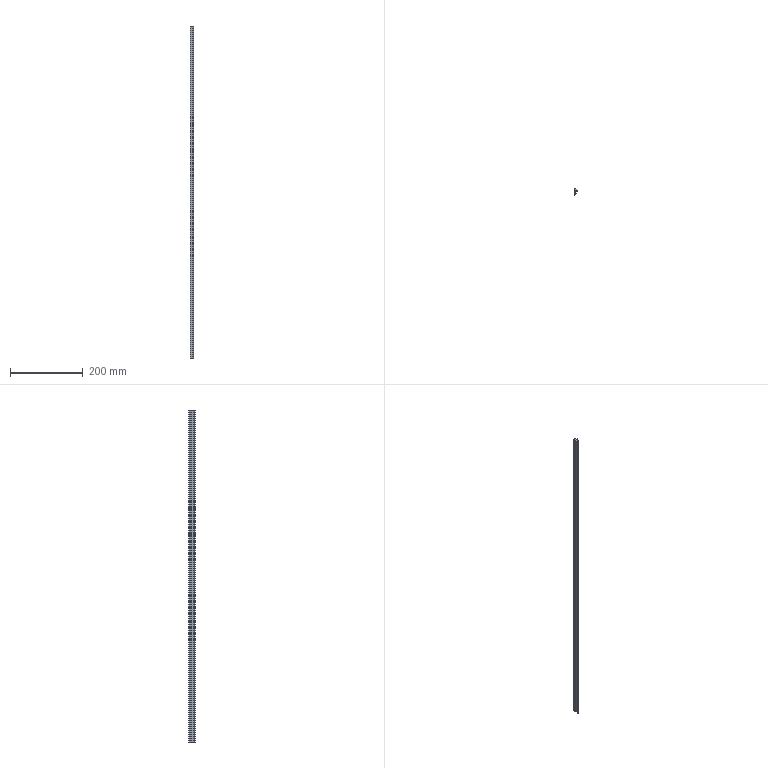Part | SolidWorks | features BaseBody 1, MoveFace 1 | 1 solid | 20 faces | box 10.8 x 17.5 x 915 mm | volume 72103 mm3 | cylinder 11 | plane 9 | commonest cylinder face diameters 1.6 x2 14 x2 0.4 x1 0.6 x1 0.8 x1 2.6 x1
STEP:
#1=CARTESIAN_POINT('',(-3.236,-11.055,815.));
#2=VERTEX_POINT('',#1);
#3=CARTESIAN_POINT('',(-4.3,-10.3,815.));
#4=VERTEX_POINT('',#3);
#5=CARTESIAN_POINT('',(-3.5,-10.3,815.));
#6=DIRECTION('',(0.,0.,-1.));
#7=DIRECTION('',(1.,0.,0.));
#8=AXIS2_PLACEMENT_3D('',#5,#6,#7);
#9=CIRCLE('',#8,0.8);
#10=EDGE_CURVE('',#2,#4,#9,.T.);
#11=ORIENTED_EDGE('',*,*,#10,.T.);
#12=CARTESIAN_POINT('',(-4.3,-10.3,-100.));
#13=VERTEX_POINT('',#12);
#14=CARTESIAN_POINT('',(-4.3,-10.3,-100.));
#15=DIRECTION('',(0.,0.,-1.));
#16=VECTOR('',#15,1000.);
#17=LINE('',#14,#16);
#18=EDGE_CURVE('',#4,#13,#17,.T.);
#19=ORIENTED_EDGE('',*,*,#18,.T.);
#20=CARTESIAN_POINT('',(-3.236,-11.055,-100.));
#21=VERTEX_POINT('',#20);
#22=CARTESIAN_POINT('',(-3.5,-10.3,-100.));
#23=DIRECTION('',(0.,0.,1.));
#24=DIRECTION('',(-1.,0.,0.));
#25=AXIS2_PLACEMENT_3D('',#22,#23,#24);
#26=CIRCLE('',#25,0.8);
#27=EDGE_CURVE('',#13,#21,#26,.T.);
#28=ORIENTED_EDGE('',*,*,#27,.T.);
#29=CARTESIAN_POINT('',(-3.236,-11.055,-100.));
#30=DIRECTION('',(0.,0.,-1.));
#31=VECTOR('',#30,1000.);
#32=LINE('',#29,#31);
#33=EDGE_CURVE('',#2,#21,#32,.T.);
#34=ORIENTED_EDGE('',*,*,#33,.F.);
#35=EDGE_LOOP('',(#11,#19,#28,#34));
#36=FACE_OUTER_BOUND('',#35,.T.);
#37=CARTESIAN_POINT('',(-3.5,-10.3,-100.));
#38=DIRECTION('',(0.,0.,-1.));
#39=DIRECTION('',(-1.,0.,0.));
#40=AXIS2_PLACEMENT_3D('',#37,#38,#39);
#41=CYLINDRICAL_SURFACE('',#40,0.8);
#42=ADVANCED_FACE('',(#36),#41,.T.);
#43=CARTESIAN_POINT('',(1.184,-6.397,-100.));
#44=VERTEX_POINT('',#43);
#45=CARTESIAN_POINT('',(-5.702,-4.29,-100.));
#46=DIRECTION('',(0.,0.,1.));
#47=DIRECTION('',(-1.,0.,0.));
#48=AXIS2_PLACEMENT_3D('',#45,#46,#47);
#49=CIRCLE('',#48,7.201);
#50=EDGE_CURVE('',#21,#44,#49,.T.);
#51=ORIENTED_EDGE('',*,*,#50,.T.);
#52=CARTESIAN_POINT('',(1.184,-6.397,815.));
#53=VERTEX_POINT('',#52);
#54=CARTESIAN_POINT('',(1.184,-6.397,-100.));
#55=DIRECTION('',(0.,0.,1.));
#56=VECTOR('',#55,1000.);
#57=LINE('',#54,#56);
#58=EDGE_CURVE('',#44,#53,#57,.T.);
#59=ORIENTED_EDGE('',*,*,#58,.T.);
#60=CARTESIAN_POINT('',(-5.702,-4.29,815.));
#61=DIRECTION('',(0.,0.,-1.));
#62=DIRECTION('',(1.,0.,0.));
#63=AXIS2_PLACEMENT_3D('',#60,#61,#62);
#64=CIRCLE('',#63,7.201);
#65=EDGE_CURVE('',#53,#2,#64,.T.);
#66=ORIENTED_EDGE('',*,*,#65,.T.);
#67=ORIENTED_EDGE('',*,*,#33,.T.);
#68=EDGE_LOOP('',(#51,#59,#66,#67));
#69=FACE_OUTER_BOUND('',#68,.T.);
#70=CARTESIAN_POINT('',(-5.702,-4.29,-100.));
#71=DIRECTION('',(0.,0.,-1.));
#72=DIRECTION('',(-1.,0.,0.));
#73=AXIS2_PLACEMENT_3D('',#70,#71,#72);
#74=CYLINDRICAL_SURFACE('',#73,7.201);
#75=ADVANCED_FACE('',(#69),#74,.T.);
#76=CARTESIAN_POINT('',(0.9,-6.,-100.));
#77=VERTEX_POINT('',#76);
#78=CARTESIAN_POINT('',(0.9,-6.3,-100.));
#79=DIRECTION('',(0.,0.,1.));
#80=DIRECTION('',(-1.,0.,0.));
#81=AXIS2_PLACEMENT_3D('',#78,#79,#80);
#82=CIRCLE('',#81,0.3);
#83=EDGE_CURVE('',#44,#77,#82,.T.);
#84=ORIENTED_EDGE('',*,*,#83,.T.);
#85=CARTESIAN_POINT('',(0.9,-6.,815.));
#86=VERTEX_POINT('',#85);
#87=CARTESIAN_POINT('',(0.9,-6.,-100.));
#88=DIRECTION('',(0.,0.,1.));
#89=VECTOR('',#88,1000.);
#90=LINE('',#87,#89);
#91=EDGE_CURVE('',#77,#86,#90,.T.);
#92=ORIENTED_EDGE('',*,*,#91,.T.);
#93=CARTESIAN_POINT('',(0.9,-6.3,815.));
#94=DIRECTION('',(0.,0.,-1.));
#95=DIRECTION('',(1.,0.,0.));
#96=AXIS2_PLACEMENT_3D('',#93,#94,#95);
#97=CIRCLE('',#96,0.3);
#98=EDGE_CURVE('',#86,#53,#97,.T.);
#99=ORIENTED_EDGE('',*,*,#98,.T.);
#100=ORIENTED_EDGE('',*,*,#58,.F.);
#101=EDGE_LOOP('',(#84,#92,#99,#100));
#102=FACE_OUTER_BOUND('',#101,.T.);
#103=CARTESIAN_POINT('',(0.9,-6.3,-100.));
#104=DIRECTION('',(0.,0.,-1.));
#105=DIRECTION('',(-1.,0.,0.));
#106=AXIS2_PLACEMENT_3D('',#103,#104,#105);
#107=CYLINDRICAL_SURFACE('',#106,0.3);
#108=ADVANCED_FACE('',(#102),#107,.T.);
#109=CARTESIAN_POINT('',(-2.5,-0.5,-100.));
#110=VERTEX_POINT('',#109);
#111=CARTESIAN_POINT('',(-2.5,-6.153,-100.));
#112=VERTEX_POINT('',#111);
#113=CARTESIAN_POINT('',(-2.5,-6.397,-100.));
#114=DIRECTION('',(0.,-1.,0.));
#115=VECTOR('',#114,1000.);
#116=LINE('',#113,#115);
#117=EDGE_CURVE('',#110,#112,#116,.T.);
#118=ORIENTED_EDGE('',*,*,#117,.F.);
#119=CARTESIAN_POINT('',(-4.2,1.695,-100.));
#120=VERTEX_POINT('',#119);
#121=CARTESIAN_POINT('',(-1.701,1.875,-100.));
#122=DIRECTION('',(0.,0.,1.));
#123=DIRECTION('',(-1.,0.,0.));
#124=AXIS2_PLACEMENT_3D('',#121,#122,#123);
#125=CIRCLE('',#124,2.506);
#126=EDGE_CURVE('',#120,#110,#125,.T.);
#127=ORIENTED_EDGE('',*,*,#126,.F.);
#128=CARTESIAN_POINT('',(-4.2,5.1,-100.));
#129=VERTEX_POINT('',#128);
#130=CARTESIAN_POINT('',(-4.2,-6.397,-100.));
#131=DIRECTION('',(0.,-1.,0.));
#132=VECTOR('',#131,1000.);
#133=LINE('',#130,#132);
#134=EDGE_CURVE('',#129,#120,#133,.T.);
#135=ORIENTED_EDGE('',*,*,#134,.F.);
#136=CARTESIAN_POINT('',(-2.892,6.4,-100.));
#137=VERTEX_POINT('',#136);
#138=CARTESIAN_POINT('',(-2.9,5.1,-100.));
#139=DIRECTION('',(0.,0.,1.));
#140=DIRECTION('',(-1.,0.,0.));
#141=AXIS2_PLACEMENT_3D('',#138,#139,#140);
#142=CIRCLE('',#141,1.3);
#143=EDGE_CURVE('',#137,#129,#142,.T.);
#144=ORIENTED_EDGE('',*,*,#143,.F.);
#145=CARTESIAN_POINT('',(0.5,5.5,-100.));
#146=VERTEX_POINT('',#145);
#147=CARTESIAN_POINT('',(-2.934,-0.5999,-100.));
#148=DIRECTION('',(0.,0.,1.));
#149=DIRECTION('',(-1.,0.,0.));
#150=AXIS2_PLACEMENT_3D('',#147,#148,#149);
#151=CIRCLE('',#150,7.);
#152=EDGE_CURVE('',#146,#137,#151,.T.);
#153=ORIENTED_EDGE('',*,*,#152,.F.);
#154=CARTESIAN_POINT('',(5.5,1.7,-100.));
#155=VERTEX_POINT('',#154);
#156=CARTESIAN_POINT('',(5.5,1.7,-100.));
#157=DIRECTION('',(-0.7962,0.6051,0.));
#158=VECTOR('',#157,1000.);
#159=LINE('',#156,#158);
#160=EDGE_CURVE('',#155,#146,#159,.T.);
#161=ORIENTED_EDGE('',*,*,#160,.F.);
#162=CARTESIAN_POINT('',(6.458,-0.2215,-100.));
#163=VERTEX_POINT('',#162);
#164=CARTESIAN_POINT('',(6.458,-0.2215,-100.));
#165=DIRECTION('',(-0.4462,0.8949,0.));
#166=VECTOR('',#165,1000.);
#167=LINE('',#164,#166);
#168=EDGE_CURVE('',#163,#155,#167,.T.);
#169=ORIENTED_EDGE('',*,*,#168,.F.);
#170=CARTESIAN_POINT('',(5.895,-0.7433,-100.));
#171=VERTEX_POINT('',#170);
#172=CARTESIAN_POINT('',(6.1,-0.4,-100.));
#173=DIRECTION('',(0.,0.,1.));
#174=DIRECTION('',(-1.,0.,0.));
#175=AXIS2_PLACEMENT_3D('',#172,#173,#174);
#176=CIRCLE('',#175,0.4);
#177=EDGE_CURVE('',#171,#163,#176,.T.);
#178=ORIENTED_EDGE('',*,*,#177,.F.);
#179=CARTESIAN_POINT('',(3.,0.,-100.));
#180=VERTEX_POINT('',#179);
#181=CARTESIAN_POINT('',(2.746,-6.995,-100.));
#182=DIRECTION('',(0.,0.,-1.));
#183=DIRECTION('',(-1.,0.,0.));
#184=AXIS2_PLACEMENT_3D('',#181,#182,#183);
#185=CIRCLE('',#184,7.);
#186=EDGE_CURVE('',#180,#171,#185,.T.);
#187=ORIENTED_EDGE('',*,*,#186,.F.);
#188=CARTESIAN_POINT('',(0.,0.,-100.));
#189=VERTEX_POINT('',#188);
#190=CARTESIAN_POINT('',(-6.814,0.,-100.));
#191=DIRECTION('',(1.,0.,0.));
#192=VECTOR('',#191,1000.);
#193=LINE('',#190,#192);
#194=EDGE_CURVE('',#189,#180,#193,.T.);
#195=ORIENTED_EDGE('',*,*,#194,.F.);
#196=CARTESIAN_POINT('',(0.,-5.8,-100.));
#197=VERTEX_POINT('',#196);
#198=CARTESIAN_POINT('',(0.,-6.397,-100.));
#199=DIRECTION('',(0.,1.,0.));
#200=VECTOR('',#199,1000.);
#201=LINE('',#198,#200);
#202=EDGE_CURVE('',#197,#189,#201,.T.);
#203=ORIENTED_EDGE('',*,*,#202,.F.);
#204=CARTESIAN_POINT('',(0.2,-6.,-100.));
#205=VERTEX_POINT('',#204);
#206=CARTESIAN_POINT('',(0.2,-5.8,-100.));
#207=DIRECTION('',(0.,0.,1.));
#208=DIRECTION('',(-1.,0.,0.));
#209=AXIS2_PLACEMENT_3D('',#206,#207,#208);
#210=CIRCLE('',#209,0.2);
#211=EDGE_CURVE('',#197,#205,#210,.T.);
#212=ORIENTED_EDGE('',*,*,#211,.T.);
#213=CARTESIAN_POINT('',(-6.814,-6.,-100.));
#214=DIRECTION('',(-1.,0.,0.));
#215=VECTOR('',#214,1000.);
#216=LINE('',#213,#215);
#217=EDGE_CURVE('',#77,#205,#216,.T.);
#218=ORIENTED_EDGE('',*,*,#217,.F.);
#219=ORIENTED_EDGE('',*,*,#83,.F.);
#220=ORIENTED_EDGE('',*,*,#50,.F.);
#221=ORIENTED_EDGE('',*,*,#27,.F.);
#222=CARTESIAN_POINT('',(-3.998,-9.674,-100.));
#223=VERTEX_POINT('',#222);
#224=CARTESIAN_POINT('',(-3.5,-10.3,-100.));
#225=DIRECTION('',(0.,0.,1.));
#226=DIRECTION('',(-1.,0.,0.));
#227=AXIS2_PLACEMENT_3D('',#224,#225,#226);
#228=CIRCLE('',#227,0.8);
#229=EDGE_CURVE('',#223,#13,#228,.T.);
#230=ORIENTED_EDGE('',*,*,#229,.F.);
#231=CARTESIAN_POINT('',(-6.814,-6.397,-100.));
#232=DIRECTION('',(0.,0.,-1.));
#233=DIRECTION('',(-1.,0.,0.));
#234=AXIS2_PLACEMENT_3D('',#231,#232,#233);
#235=CIRCLE('',#234,4.321);
#236=EDGE_CURVE('',#112,#223,#235,.T.);
#237=ORIENTED_EDGE('',*,*,#236,.F.);
#238=EDGE_LOOP('',(#118,#127,#135,#144,#153,#161,#169,#178,#187,#195,#203,#212,#218,#219,#220,#221,#230,#237));
#239=FACE_OUTER_BOUND('',#238,.T.);
#240=CARTESIAN_POINT('',(-6.814,-6.397,-100.));
#241=DIRECTION('',(0.,0.,1.));
#242=DIRECTION('',(1.,0.,0.));
#243=AXIS2_PLACEMENT_3D('',#240,#241,#242);
#244=PLANE('',#243);
#245=ADVANCED_FACE('',(#239),#244,.F.);
#246=ORIENTED_EDGE('',*,*,#18,.F.);
#247=CARTESIAN_POINT('',(-3.998,-9.674,815.));
#248=VERTEX_POINT('',#247);
#249=CARTESIAN_POINT('',(-3.5,-10.3,815.));
#250=DIRECTION('',(0.,0.,-1.));
#251=DIRECTION('',(1.,0.,0.));
#252=AXIS2_PLACEMENT_3D('',#249,#250,#251);
#253=CIRCLE('',#252,0.8);
#254=EDGE_CURVE('',#4,#248,#253,.T.);
#255=ORIENTED_EDGE('',*,*,#254,.T.);
#256=CARTESIAN_POINT('',(-3.998,-9.674,-100.));
#257=DIRECTION('',(0.,0.,-1.));
#258=VECTOR('',#257,1000.);
#259=LINE('',#256,#258);
#260=EDGE_CURVE('',#248,#223,#259,.T.);
#261=ORIENTED_EDGE('',*,*,#260,.T.);
#262=ORIENTED_EDGE('',*,*,#229,.T.);
#263=EDGE_LOOP('',(#246,#255,#261,#262));
#264=FACE_OUTER_BOUND('',#263,.T.);
#265=CARTESIAN_POINT('',(-3.5,-10.3,-100.));
#266=DIRECTION('',(0.,0.,-1.));
#267=DIRECTION('',(-1.,0.,0.));
#268=AXIS2_PLACEMENT_3D('',#265,#266,#267);
#269=CYLINDRICAL_SURFACE('',#268,0.8);
#270=ADVANCED_FACE('',(#264),#269,.T.);
#271=CARTESIAN_POINT('',(-4.2,1.695,815.));
#272=VERTEX_POINT('',#271);
#273=CARTESIAN_POINT('',(-2.5,-0.5,815.));
#274=VERTEX_POINT('',#273);
#275=CARTESIAN_POINT('',(-1.701,1.875,815.));
#276=DIRECTION('',(0.,0.,1.));
#277=DIRECTION('',(1.,0.,0.));
#278=AXIS2_PLACEMENT_3D('',#275,#276,#277);
#279=CIRCLE('',#278,2.506);
#280=EDGE_CURVE('',#272,#274,#279,.T.);
#281=ORIENTED_EDGE('',*,*,#280,.T.);
#282=CARTESIAN_POINT('',(-2.5,-6.153,815.));
#283=VERTEX_POINT('',#282);
#284=CARTESIAN_POINT('',(-2.5,-6.397,815.));
#285=DIRECTION('',(0.,-1.,0.));
#286=VECTOR('',#285,1000.);
#287=LINE('',#284,#286);
#288=EDGE_CURVE('',#274,#283,#287,.T.);
#289=ORIENTED_EDGE('',*,*,#288,.T.);
#290=CARTESIAN_POINT('',(-6.814,-6.397,815.));
#291=DIRECTION('',(0.,0.,-1.));
#292=DIRECTION('',(1.,0.,0.));
#293=AXIS2_PLACEMENT_3D('',#290,#291,#292);
#294=CIRCLE('',#293,4.321);
#295=EDGE_CURVE('',#283,#248,#294,.T.);
#296=ORIENTED_EDGE('',*,*,#295,.T.);
#297=ORIENTED_EDGE('',*,*,#254,.F.);
#298=ORIENTED_EDGE('',*,*,#10,.F.);
#299=ORIENTED_EDGE('',*,*,#65,.F.);
#300=ORIENTED_EDGE('',*,*,#98,.F.);
#301=CARTESIAN_POINT('',(0.2,-6.,815.));
#302=VERTEX_POINT('',#301);
#303=CARTESIAN_POINT('',(-6.814,-6.,815.));
#304=DIRECTION('',(-1.,0.,0.));
#305=VECTOR('',#304,1000.);
#306=LINE('',#303,#305);
#307=EDGE_CURVE('',#86,#302,#306,.T.);
#308=ORIENTED_EDGE('',*,*,#307,.T.);
#309=CARTESIAN_POINT('',(0.,-5.8,815.));
#310=VERTEX_POINT('',#309);
#311=CARTESIAN_POINT('',(0.2,-5.8,815.));
#312=DIRECTION('',(0.,0.,-1.));
#313=DIRECTION('',(1.,0.,0.));
#314=AXIS2_PLACEMENT_3D('',#311,#312,#313);
#315=CIRCLE('',#314,0.2);
#316=EDGE_CURVE('',#302,#310,#315,.T.);
#317=ORIENTED_EDGE('',*,*,#316,.T.);
#318=CARTESIAN_POINT('',(0.,0.,815.));
#319=VERTEX_POINT('',#318);
#320=CARTESIAN_POINT('',(0.,-6.397,815.));
#321=DIRECTION('',(0.,1.,0.));
#322=VECTOR('',#321,1000.);
#323=LINE('',#320,#322);
#324=EDGE_CURVE('',#310,#319,#323,.T.);
#325=ORIENTED_EDGE('',*,*,#324,.T.);
#326=CARTESIAN_POINT('',(3.,0.,815.));
#327=VERTEX_POINT('',#326);
#328=CARTESIAN_POINT('',(-6.814,0.,815.));
#329=DIRECTION('',(1.,0.,0.));
#330=VECTOR('',#329,1000.);
#331=LINE('',#328,#330);
#332=EDGE_CURVE('',#319,#327,#331,.T.);
#333=ORIENTED_EDGE('',*,*,#332,.T.);
#334=CARTESIAN_POINT('',(5.895,-0.7433,815.));
#335=VERTEX_POINT('',#334);
#336=CARTESIAN_POINT('',(2.746,-6.995,815.));
#337=DIRECTION('',(0.,0.,-1.));
#338=DIRECTION('',(1.,0.,0.));
#339=AXIS2_PLACEMENT_3D('',#336,#337,#338);
#340=CIRCLE('',#339,7.);
#341=EDGE_CURVE('',#327,#335,#340,.T.);
#342=ORIENTED_EDGE('',*,*,#341,.T.);
#343=CARTESIAN_POINT('',(6.458,-0.2215,815.));
#344=VERTEX_POINT('',#343);
#345=CARTESIAN_POINT('',(6.1,-0.4,815.));
#346=DIRECTION('',(0.,0.,-1.));
#347=DIRECTION('',(1.,0.,0.));
#348=AXIS2_PLACEMENT_3D('',#345,#346,#347);
#349=CIRCLE('',#348,0.4);
#350=EDGE_CURVE('',#344,#335,#349,.T.);
#351=ORIENTED_EDGE('',*,*,#350,.F.);
#352=CARTESIAN_POINT('',(5.5,1.7,815.));
#353=VERTEX_POINT('',#352);
#354=CARTESIAN_POINT('',(6.282,0.1323,815.));
#355=DIRECTION('',(-0.4462,0.8949,0.));
#356=VECTOR('',#355,1000.);
#357=LINE('',#354,#356);
#358=EDGE_CURVE('',#344,#353,#357,.T.);
#359=ORIENTED_EDGE('',*,*,#358,.T.);
#360=CARTESIAN_POINT('',(0.5,5.5,815.));
#361=VERTEX_POINT('',#360);
#362=CARTESIAN_POINT('',(1.595,4.668,815.));
#363=DIRECTION('',(-0.7962,0.6051,0.));
#364=VECTOR('',#363,1000.);
#365=LINE('',#362,#364);
#366=EDGE_CURVE('',#353,#361,#365,.T.);
#367=ORIENTED_EDGE('',*,*,#366,.T.);
#368=CARTESIAN_POINT('',(-2.892,6.4,815.));
#369=VERTEX_POINT('',#368);
#370=CARTESIAN_POINT('',(-2.934,-0.5999,815.));
#371=DIRECTION('',(0.,0.,1.));
#372=DIRECTION('',(1.,0.,0.));
#373=AXIS2_PLACEMENT_3D('',#370,#371,#372);
#374=CIRCLE('',#373,7.);
#375=EDGE_CURVE('',#361,#369,#374,.T.);
#376=ORIENTED_EDGE('',*,*,#375,.T.);
#377=CARTESIAN_POINT('',(-4.2,5.1,815.));
#378=VERTEX_POINT('',#377);
#379=CARTESIAN_POINT('',(-2.9,5.1,815.));
#380=DIRECTION('',(0.,0.,1.));
#381=DIRECTION('',(1.,0.,0.));
#382=AXIS2_PLACEMENT_3D('',#379,#380,#381);
#383=CIRCLE('',#382,1.3);
#384=EDGE_CURVE('',#369,#378,#383,.T.);
#385=ORIENTED_EDGE('',*,*,#384,.T.);
#386=CARTESIAN_POINT('',(-4.2,-6.397,815.));
#387=DIRECTION('',(0.,-1.,0.));
#388=VECTOR('',#387,1000.);
#389=LINE('',#386,#388);
#390=EDGE_CURVE('',#378,#272,#389,.T.);
#391=ORIENTED_EDGE('',*,*,#390,.T.);
#392=EDGE_LOOP('',(#281,#289,#296,#297,#298,#299,#300,#308,#317,#325,#333,#342,#351,#359,#367,#376,#385,#391));
#393=FACE_OUTER_BOUND('',#392,.T.);
#394=CARTESIAN_POINT('',(-6.814,-6.397,815.));
#395=DIRECTION('',(0.,0.,1.));
#396=DIRECTION('',(1.,0.,0.));
#397=AXIS2_PLACEMENT_3D('',#394,#395,#396);
#398=PLANE('',#397);
#399=ADVANCED_FACE('',(#393),#398,.T.);
#400=ORIENTED_EDGE('',*,*,#217,.T.);
#401=CARTESIAN_POINT('',(0.2,-6.,-100.));
#402=DIRECTION('',(0.,0.,1.));
#403=VECTOR('',#402,1000.);
#404=LINE('',#401,#403);
#405=EDGE_CURVE('',#205,#302,#404,.T.);
#406=ORIENTED_EDGE('',*,*,#405,.T.);
#407=ORIENTED_EDGE('',*,*,#307,.F.);
#408=ORIENTED_EDGE('',*,*,#91,.F.);
#409=EDGE_LOOP('',(#400,#406,#407,#408));
#410=FACE_OUTER_BOUND('',#409,.T.);
#411=CARTESIAN_POINT('',(0.9,-6.,-100.));
#412=DIRECTION('',(0.,1.,0.));
#413=DIRECTION('',(0.,0.,1.));
#414=AXIS2_PLACEMENT_3D('',#411,#412,#413);
#415=PLANE('',#414);
#416=ADVANCED_FACE('',(#410),#415,.T.);
#417=CARTESIAN_POINT('',(-2.5,-6.153,-100.));
#418=DIRECTION('',(0.,0.,1.));
#419=VECTOR('',#418,1000.);
#420=LINE('',#417,#419);
#421=EDGE_CURVE('',#112,#283,#420,.T.);
#422=ORIENTED_EDGE('',*,*,#421,.F.);
#423=ORIENTED_EDGE('',*,*,#236,.T.);
#424=ORIENTED_EDGE('',*,*,#260,.F.);
#425=ORIENTED_EDGE('',*,*,#295,.F.);
#426=EDGE_LOOP('',(#422,#423,#424,#425));
#427=FACE_OUTER_BOUND('',#426,.T.);
#428=CARTESIAN_POINT('',(-6.814,-6.397,-100.));
#429=DIRECTION('',(0.,0.,-1.));
#430=DIRECTION('',(-1.,0.,0.));
#431=AXIS2_PLACEMENT_3D('',#428,#429,#430);
#432=CYLINDRICAL_SURFACE('',#431,4.321);
#433=ADVANCED_FACE('',(#427),#432,.F.);
#434=ORIENTED_EDGE('',*,*,#117,.T.);
#435=ORIENTED_EDGE('',*,*,#421,.T.);
#436=ORIENTED_EDGE('',*,*,#288,.F.);
#437=CARTESIAN_POINT('',(-2.5,-0.5,-100.));
#438=DIRECTION('',(0.,0.,-1.));
#439=VECTOR('',#438,1000.);
#440=LINE('',#437,#439);
#441=EDGE_CURVE('',#274,#110,#440,.T.);
#442=ORIENTED_EDGE('',*,*,#441,.T.);
#443=EDGE_LOOP('',(#434,#435,#436,#442));
#444=FACE_OUTER_BOUND('',#443,.T.);
#445=CARTESIAN_POINT('',(-2.5,-0.5,-100.));
#446=DIRECTION('',(-1.,0.,0.));
#447=DIRECTION('',(0.,0.,1.));
#448=AXIS2_PLACEMENT_3D('',#445,#446,#447);
#449=PLANE('',#448);
#450=ADVANCED_FACE('',(#444),#449,.T.);
#451=ORIENTED_EDGE('',*,*,#126,.T.);
#452=ORIENTED_EDGE('',*,*,#441,.F.);
#453=ORIENTED_EDGE('',*,*,#280,.F.);
#454=CARTESIAN_POINT('',(-4.2,1.695,-100.));
#455=DIRECTION('',(0.,0.,-1.));
#456=VECTOR('',#455,1000.);
#457=LINE('',#454,#456);
#458=EDGE_CURVE('',#272,#120,#457,.T.);
#459=ORIENTED_EDGE('',*,*,#458,.T.);
#460=EDGE_LOOP('',(#451,#452,#453,#459));
#461=FACE_OUTER_BOUND('',#460,.T.);
#462=CARTESIAN_POINT('',(-1.701,1.875,-100.));
#463=DIRECTION('',(0.,0.,-1.));
#464=DIRECTION('',(-1.,0.,0.));
#465=AXIS2_PLACEMENT_3D('',#462,#463,#464);
#466=CYLINDRICAL_SURFACE('',#465,2.506);
#467=ADVANCED_FACE('',(#461),#466,.T.);
#468=ORIENTED_EDGE('',*,*,#134,.T.);
#469=ORIENTED_EDGE('',*,*,#458,.F.);
#470=ORIENTED_EDGE('',*,*,#390,.F.);
#471=CARTESIAN_POINT('',(-4.2,5.1,-100.));
#472=DIRECTION('',(0.,0.,-1.));
#473=VECTOR('',#472,1000.);
#474=LINE('',#471,#473);
#475=EDGE_CURVE('',#378,#129,#474,.T.);
#476=ORIENTED_EDGE('',*,*,#475,.T.);
#477=EDGE_LOOP('',(#468,#469,#470,#476));
#478=FACE_OUTER_BOUND('',#477,.T.);
#479=CARTESIAN_POINT('',(-4.2,5.1,-100.));
#480=DIRECTION('',(-1.,0.,0.));
#481=DIRECTION('',(0.,0.,1.));
#482=AXIS2_PLACEMENT_3D('',#479,#480,#481);
#483=PLANE('',#482);
#484=ADVANCED_FACE('',(#478),#483,.T.);
#485=ORIENTED_EDGE('',*,*,#143,.T.);
#486=ORIENTED_EDGE('',*,*,#475,.F.);
#487=ORIENTED_EDGE('',*,*,#384,.F.);
#488=CARTESIAN_POINT('',(-2.892,6.4,-100.));
#489=DIRECTION('',(0.,0.,-1.));
#490=VECTOR('',#489,1000.);
#491=LINE('',#488,#490);
#492=EDGE_CURVE('',#369,#137,#491,.T.);
#493=ORIENTED_EDGE('',*,*,#492,.T.);
#494=EDGE_LOOP('',(#485,#486,#487,#493));
#495=FACE_OUTER_BOUND('',#494,.T.);
#496=CARTESIAN_POINT('',(-2.9,5.1,-100.));
#497=DIRECTION('',(0.,0.,-1.));
#498=DIRECTION('',(-1.,0.,0.));
#499=AXIS2_PLACEMENT_3D('',#496,#497,#498);
#500=CYLINDRICAL_SURFACE('',#499,1.3);
#501=ADVANCED_FACE('',(#495),#500,.T.);
#502=ORIENTED_EDGE('',*,*,#152,.T.);
#503=ORIENTED_EDGE('',*,*,#492,.F.);
#504=ORIENTED_EDGE('',*,*,#375,.F.);
#505=CARTESIAN_POINT('',(0.5,5.5,-100.));
#506=DIRECTION('',(0.,0.,-1.));
#507=VECTOR('',#506,1000.);
#508=LINE('',#505,#507);
#509=EDGE_CURVE('',#361,#146,#508,.T.);
#510=ORIENTED_EDGE('',*,*,#509,.T.);
#511=EDGE_LOOP('',(#502,#503,#504,#510));
#512=FACE_OUTER_BOUND('',#511,.T.);
#513=CARTESIAN_POINT('',(-2.934,-0.5999,-100.));
#514=DIRECTION('',(0.,0.,-1.));
#515=DIRECTION('',(-1.,0.,0.));
#516=AXIS2_PLACEMENT_3D('',#513,#514,#515);
#517=CYLINDRICAL_SURFACE('',#516,7.);
#518=ADVANCED_FACE('',(#512),#517,.T.);
#519=ORIENTED_EDGE('',*,*,#160,.T.);
#520=ORIENTED_EDGE('',*,*,#509,.F.);
#521=ORIENTED_EDGE('',*,*,#366,.F.);
#522=CARTESIAN_POINT('',(5.5,1.7,-100.));
#523=DIRECTION('',(0.,0.,-1.));
#524=VECTOR('',#523,1000.);
#525=LINE('',#522,#524);
#526=EDGE_CURVE('',#353,#155,#525,.T.);
#527=ORIENTED_EDGE('',*,*,#526,.T.);
#528=EDGE_LOOP('',(#519,#520,#521,#527));
#529=FACE_OUTER_BOUND('',#528,.T.);
#530=CARTESIAN_POINT('',(5.5,1.7,-100.));
#531=DIRECTION('',(0.6051,0.7962,0.));
#532=DIRECTION('',(-0.7962,0.6051,0.));
#533=AXIS2_PLACEMENT_3D('',#530,#531,#532);
#534=PLANE('',#533);
#535=ADVANCED_FACE('',(#529),#534,.T.);
#536=ORIENTED_EDGE('',*,*,#168,.T.);
#537=ORIENTED_EDGE('',*,*,#526,.F.);
#538=ORIENTED_EDGE('',*,*,#358,.F.);
#539=CARTESIAN_POINT('',(6.458,-0.2215,-100.));
#540=DIRECTION('',(0.,0.,-1.));
#541=VECTOR('',#540,1000.);
#542=LINE('',#539,#541);
#543=EDGE_CURVE('',#344,#163,#542,.T.);
#544=ORIENTED_EDGE('',*,*,#543,.T.);
#545=EDGE_LOOP('',(#536,#537,#538,#544));
#546=FACE_OUTER_BOUND('',#545,.T.);
#547=CARTESIAN_POINT('',(6.458,-0.2215,-100.));
#548=DIRECTION('',(0.8949,0.4462,0.));
#549=DIRECTION('',(-0.4462,0.8949,0.));
#550=AXIS2_PLACEMENT_3D('',#547,#548,#549);
#551=PLANE('',#550);
#552=ADVANCED_FACE('',(#546),#551,.T.);
#553=CARTESIAN_POINT('',(3.,0.,-100.));
#554=DIRECTION('',(0.,0.,1.));
#555=VECTOR('',#554,1000.);
#556=LINE('',#553,#555);
#557=EDGE_CURVE('',#180,#327,#556,.T.);
#558=ORIENTED_EDGE('',*,*,#557,.F.);
#559=ORIENTED_EDGE('',*,*,#186,.T.);
#560=CARTESIAN_POINT('',(5.895,-0.7433,-100.));
#561=DIRECTION('',(0.,0.,-1.));
#562=VECTOR('',#561,1000.);
#563=LINE('',#560,#562);
#564=EDGE_CURVE('',#335,#171,#563,.T.);
#565=ORIENTED_EDGE('',*,*,#564,.F.);
#566=ORIENTED_EDGE('',*,*,#341,.F.);
#567=EDGE_LOOP('',(#558,#559,#565,#566));
#568=FACE_OUTER_BOUND('',#567,.T.);
#569=CARTESIAN_POINT('',(2.746,-6.995,-100.));
#570=DIRECTION('',(0.,0.,-1.));
#571=DIRECTION('',(-1.,0.,0.));
#572=AXIS2_PLACEMENT_3D('',#569,#570,#571);
#573=CYLINDRICAL_SURFACE('',#572,7.);
#574=ADVANCED_FACE('',(#568),#573,.F.);
#575=ORIENTED_EDGE('',*,*,#194,.T.);
#576=ORIENTED_EDGE('',*,*,#557,.T.);
#577=ORIENTED_EDGE('',*,*,#332,.F.);
#578=CARTESIAN_POINT('',(0.,0.,-100.));
#579=DIRECTION('',(0.,0.,-1.));
#580=VECTOR('',#579,1000.);
#581=LINE('',#578,#580);
#582=EDGE_CURVE('',#319,#189,#581,.T.);
#583=ORIENTED_EDGE('',*,*,#582,.T.);
#584=EDGE_LOOP('',(#575,#576,#577,#583));
#585=FACE_OUTER_BOUND('',#584,.T.);
#586=CARTESIAN_POINT('',(0.,0.,-100.));
#587=DIRECTION('',(0.,-1.,0.));
#588=DIRECTION('',(0.,0.,-1.));
#589=AXIS2_PLACEMENT_3D('',#586,#587,#588);
#590=PLANE('',#589);
#591=ADVANCED_FACE('',(#585),#590,.T.);
#592=ORIENTED_EDGE('',*,*,#202,.T.);
#593=ORIENTED_EDGE('',*,*,#582,.F.);
#594=ORIENTED_EDGE('',*,*,#324,.F.);
#595=CARTESIAN_POINT('',(0.,-5.8,-100.));
#596=DIRECTION('',(0.,0.,-1.));
#597=VECTOR('',#596,1000.);
#598=LINE('',#595,#597);
#599=EDGE_CURVE('',#310,#197,#598,.T.);
#600=ORIENTED_EDGE('',*,*,#599,.T.);
#601=EDGE_LOOP('',(#592,#593,#594,#600));
#602=FACE_OUTER_BOUND('',#601,.T.);
#603=CARTESIAN_POINT('',(0.,-5.8,-100.));
#604=DIRECTION('',(1.,0.,0.));
#605=DIRECTION('',(0.,0.,-1.));
#606=AXIS2_PLACEMENT_3D('',#603,#604,#605);
#607=PLANE('',#606);
#608=ADVANCED_FACE('',(#602),#607,.T.);
#609=ORIENTED_EDGE('',*,*,#405,.F.);
#610=ORIENTED_EDGE('',*,*,#211,.F.);
#611=ORIENTED_EDGE('',*,*,#599,.F.);
#612=ORIENTED_EDGE('',*,*,#316,.F.);
#613=EDGE_LOOP('',(#609,#610,#611,#612));
#614=FACE_OUTER_BOUND('',#613,.T.);
#615=CARTESIAN_POINT('',(0.2,-5.8,-100.));
#616=DIRECTION('',(0.,0.,-1.));
#617=DIRECTION('',(-1.,0.,0.));
#618=AXIS2_PLACEMENT_3D('',#615,#616,#617);
#619=CYLINDRICAL_SURFACE('',#618,0.2);
#620=ADVANCED_FACE('',(#614),#619,.F.);
#621=ORIENTED_EDGE('',*,*,#177,.T.);
#622=ORIENTED_EDGE('',*,*,#543,.F.);
#623=ORIENTED_EDGE('',*,*,#350,.T.);
#624=ORIENTED_EDGE('',*,*,#564,.T.);
#625=EDGE_LOOP('',(#621,#622,#623,#624));
#626=FACE_OUTER_BOUND('',#625,.T.);
#627=CARTESIAN_POINT('',(6.1,-0.4,-100.));
#628=DIRECTION('',(0.,0.,-1.));
#629=DIRECTION('',(-1.,0.,0.));
#630=AXIS2_PLACEMENT_3D('',#627,#628,#629);
#631=CYLINDRICAL_SURFACE('',#630,0.4);
#632=ADVANCED_FACE('',(#626),#631,.T.);
#633=CLOSED_SHELL('',(#42,#75,#108,#245,#270,#399,#416,#433,#450,#467,#484,#501,#518,#535,#552,#574,#591,#608,#620,#632));
#634=MANIFOLD_SOLID_BREP('',#633);
#635=CARTESIAN_POINT('',(0.,0.,0.));
#636=DIRECTION('',(0.,0.,1.));
#637=DIRECTION('',(1.,0.,0.));
#638=AXIS2_PLACEMENT_3D('',#635,#636,#637);
#639=(LENGTH_UNIT()NAMED_UNIT(*)SI_UNIT(.MILLI.,.METRE.));
#640=UNCERTAINTY_MEASURE_WITH_UNIT(LENGTH_MEASURE(0.00001),#639,'','');
#641=(NAMED_UNIT(*)PLANE_ANGLE_UNIT()SI_UNIT($,.RADIAN.));
#642=(NAMED_UNIT(*)SI_UNIT($,.STERADIAN.)SOLID_ANGLE_UNIT());
#643=(GEOMETRIC_REPRESENTATION_CONTEXT(3)GLOBAL_UNCERTAINTY_ASSIGNED_CONTEXT((#640))GLOBAL_UNIT_ASSIGNED_CONTEXT((#639,#641,#642))REPRESENTATION_CONTEXT('',''));
#644=ADVANCED_BREP_SHAPE_REPRESENTATION('',(#634,#638),#643);